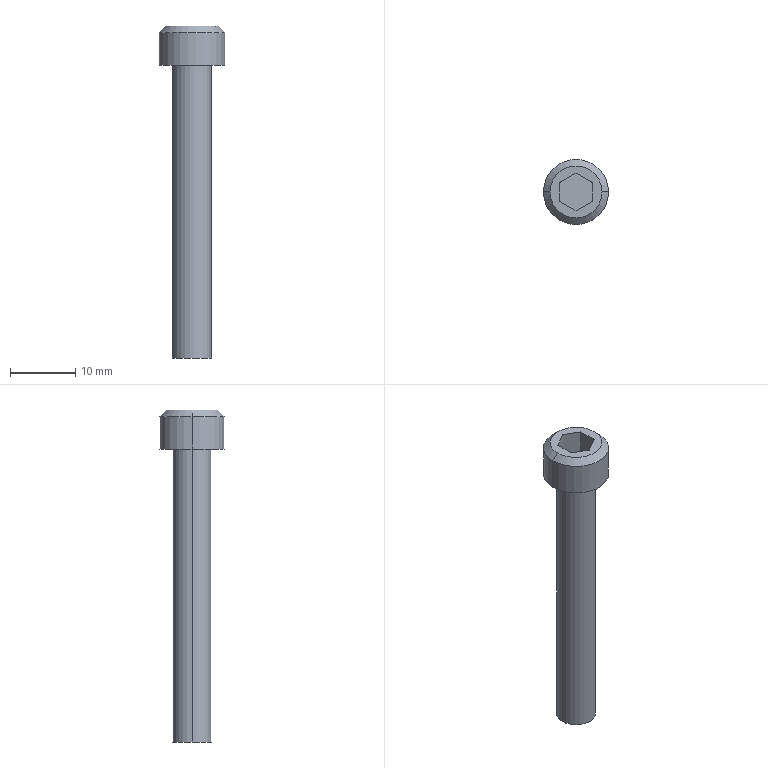Part | SolidWorks | features ICE 2, Chamfer 1, Extrusion 1 | 1 solid | 16 faces | box 10 x 10 x 51 mm | volume 1642 mm3 | plane 10 | cylinder 4 | cone 2 | commonest cylinder face diameters 6 x2 10 x2
STEP:
#1=CARTESIAN_POINT('',(-3.,0.,-45.));
#2=VERTEX_POINT('',#1);
#3=CARTESIAN_POINT('',(3.,0.,-45.));
#4=VERTEX_POINT('',#3);
#5=CARTESIAN_POINT('',(0.,0.,-45.));
#6=DIRECTION('',(0.,0.,-1.));
#7=DIRECTION('',(-1.,0.,0.));
#8=AXIS2_PLACEMENT_3D('',#5,#6,#7);
#9=CIRCLE('',#8,3.);
#10=EDGE_CURVE('',#2,#4,#9,.T.);
#11=ORIENTED_EDGE('',*,*,#10,.F.);
#12=CARTESIAN_POINT('',(-3.,0.,0.));
#13=VERTEX_POINT('',#12);
#14=CARTESIAN_POINT('',(-3.,0.,-45.));
#15=DIRECTION('',(0.,0.,1.));
#16=VECTOR('',#15,1000.);
#17=LINE('',#14,#16);
#18=EDGE_CURVE('',#2,#13,#17,.T.);
#19=ORIENTED_EDGE('',*,*,#18,.T.);
#20=CARTESIAN_POINT('',(3.,0.,0.));
#21=VERTEX_POINT('',#20);
#22=CARTESIAN_POINT('',(0.,0.,0.));
#23=DIRECTION('',(0.,0.,-1.));
#24=DIRECTION('',(1.,0.,0.));
#25=AXIS2_PLACEMENT_3D('',#22,#23,#24);
#26=CIRCLE('',#25,3.);
#27=EDGE_CURVE('',#13,#21,#26,.T.);
#28=ORIENTED_EDGE('',*,*,#27,.T.);
#29=CARTESIAN_POINT('',(3.,0.,-45.));
#30=DIRECTION('',(0.,0.,1.));
#31=VECTOR('',#30,1000.);
#32=LINE('',#29,#31);
#33=EDGE_CURVE('',#4,#21,#32,.T.);
#34=ORIENTED_EDGE('',*,*,#33,.F.);
#35=EDGE_LOOP('',(#11,#19,#28,#34));
#36=FACE_OUTER_BOUND('',#35,.T.);
#37=CARTESIAN_POINT('',(0.,0.,-45.));
#38=DIRECTION('',(0.,0.,1.));
#39=DIRECTION('',(1.,0.,0.));
#40=AXIS2_PLACEMENT_3D('',#37,#38,#39);
#41=CYLINDRICAL_SURFACE('',#40,3.);
#42=ADVANCED_FACE('',(#36),#41,.T.);
#43=CARTESIAN_POINT('',(4.,0.,6.));
#44=VERTEX_POINT('',#43);
#45=CARTESIAN_POINT('',(-4.,0.,6.));
#46=VERTEX_POINT('',#45);
#47=CARTESIAN_POINT('',(0.,0.,6.));
#48=DIRECTION('',(0.,0.,1.));
#49=DIRECTION('',(1.,0.,0.));
#50=AXIS2_PLACEMENT_3D('',#47,#48,#49);
#51=CIRCLE('',#50,4.);
#52=EDGE_CURVE('',#44,#46,#51,.T.);
#53=ORIENTED_EDGE('',*,*,#52,.F.);
#54=CARTESIAN_POINT('',(5.,0.,5.));
#55=VERTEX_POINT('',#54);
#56=CARTESIAN_POINT('',(4.,0.,6.));
#57=DIRECTION('',(0.7071,0.,-0.7071));
#58=VECTOR('',#57,1000.);
#59=LINE('',#56,#58);
#60=EDGE_CURVE('',#44,#55,#59,.T.);
#61=ORIENTED_EDGE('',*,*,#60,.T.);
#62=CARTESIAN_POINT('',(-5.,0.,5.));
#63=VERTEX_POINT('',#62);
#64=CARTESIAN_POINT('',(0.,0.,5.));
#65=DIRECTION('',(0.,0.,-1.));
#66=DIRECTION('',(1.,0.,0.));
#67=AXIS2_PLACEMENT_3D('',#64,#65,#66);
#68=CIRCLE('',#67,5.);
#69=EDGE_CURVE('',#63,#55,#68,.T.);
#70=ORIENTED_EDGE('',*,*,#69,.F.);
#71=CARTESIAN_POINT('',(-4.,0.,6.));
#72=DIRECTION('',(-0.7071,0.,-0.7071));
#73=VECTOR('',#72,1000.);
#74=LINE('',#71,#73);
#75=EDGE_CURVE('',#46,#63,#74,.T.);
#76=ORIENTED_EDGE('',*,*,#75,.F.);
#77=EDGE_LOOP('',(#53,#61,#70,#76));
#78=FACE_OUTER_BOUND('',#77,.T.);
#79=CARTESIAN_POINT('',(0.,0.,6.));
#80=DIRECTION('',(0.,0.,-1.));
#81=DIRECTION('',(-1.,0.,0.));
#82=AXIS2_PLACEMENT_3D('',#79,#80,#81);
#83=CONICAL_SURFACE('',#82,4.,0.7854);
#84=ADVANCED_FACE('',(#78),#83,.T.);
#85=ORIENTED_EDGE('',*,*,#69,.T.);
#86=CARTESIAN_POINT('',(5.,0.,0.));
#87=VERTEX_POINT('',#86);
#88=CARTESIAN_POINT('',(5.,0.,6.));
#89=DIRECTION('',(0.,0.,-1.));
#90=VECTOR('',#89,1000.);
#91=LINE('',#88,#90);
#92=EDGE_CURVE('',#55,#87,#91,.T.);
#93=ORIENTED_EDGE('',*,*,#92,.T.);
#94=CARTESIAN_POINT('',(-5.,0.,0.));
#95=VERTEX_POINT('',#94);
#96=CARTESIAN_POINT('',(0.,0.,0.));
#97=DIRECTION('',(0.,0.,1.));
#98=DIRECTION('',(1.,0.,0.));
#99=AXIS2_PLACEMENT_3D('',#96,#97,#98);
#100=CIRCLE('',#99,5.);
#101=EDGE_CURVE('',#87,#95,#100,.T.);
#102=ORIENTED_EDGE('',*,*,#101,.T.);
#103=CARTESIAN_POINT('',(-5.,0.,6.));
#104=DIRECTION('',(0.,0.,-1.));
#105=VECTOR('',#104,1000.);
#106=LINE('',#103,#105);
#107=EDGE_CURVE('',#63,#95,#106,.T.);
#108=ORIENTED_EDGE('',*,*,#107,.F.);
#109=EDGE_LOOP('',(#85,#93,#102,#108));
#110=FACE_OUTER_BOUND('',#109,.T.);
#111=CARTESIAN_POINT('',(0.,0.,6.));
#112=DIRECTION('',(0.,0.,-1.));
#113=DIRECTION('',(-1.,0.,0.));
#114=AXIS2_PLACEMENT_3D('',#111,#112,#113);
#115=CYLINDRICAL_SURFACE('',#114,5.);
#116=ADVANCED_FACE('',(#110),#115,.T.);
#117=CARTESIAN_POINT('',(0.,0.,0.));
#118=DIRECTION('',(0.,0.,1.));
#119=DIRECTION('',(1.,0.,0.));
#120=AXIS2_PLACEMENT_3D('',#117,#118,#119);
#121=CIRCLE('',#120,5.);
#122=EDGE_CURVE('',#95,#87,#121,.T.);
#123=ORIENTED_EDGE('',*,*,#122,.F.);
#124=ORIENTED_EDGE('',*,*,#101,.F.);
#125=EDGE_LOOP('',(#123,#124));
#126=FACE_OUTER_BOUND('',#125,.T.);
#127=CARTESIAN_POINT('',(0.,0.,0.));
#128=DIRECTION('',(0.,0.,-1.));
#129=DIRECTION('',(1.,0.,0.));
#130=AXIS2_PLACEMENT_3D('',#127,#128,#129);
#131=CIRCLE('',#130,3.);
#132=EDGE_CURVE('',#21,#13,#131,.T.);
#133=ORIENTED_EDGE('',*,*,#132,.F.);
#134=ORIENTED_EDGE('',*,*,#27,.F.);
#135=EDGE_LOOP('',(#133,#134));
#136=FACE_BOUND('',#135,.T.);
#137=CARTESIAN_POINT('',(0.,0.,0.));
#138=DIRECTION('',(0.,0.,1.));
#139=DIRECTION('',(1.,0.,0.));
#140=AXIS2_PLACEMENT_3D('',#137,#138,#139);
#141=PLANE('',#140);
#142=ADVANCED_FACE('',(#126,#136),#141,.F.);
#143=ORIENTED_EDGE('',*,*,#92,.F.);
#144=CARTESIAN_POINT('',(0.,0.,5.));
#145=DIRECTION('',(0.,0.,-1.));
#146=DIRECTION('',(1.,0.,0.));
#147=AXIS2_PLACEMENT_3D('',#144,#145,#146);
#148=CIRCLE('',#147,5.);
#149=EDGE_CURVE('',#55,#63,#148,.T.);
#150=ORIENTED_EDGE('',*,*,#149,.T.);
#151=ORIENTED_EDGE('',*,*,#107,.T.);
#152=ORIENTED_EDGE('',*,*,#122,.T.);
#153=EDGE_LOOP('',(#143,#150,#151,#152));
#154=FACE_OUTER_BOUND('',#153,.T.);
#155=CARTESIAN_POINT('',(0.,0.,6.));
#156=DIRECTION('',(0.,0.,-1.));
#157=DIRECTION('',(-1.,0.,0.));
#158=AXIS2_PLACEMENT_3D('',#155,#156,#157);
#159=CYLINDRICAL_SURFACE('',#158,5.);
#160=ADVANCED_FACE('',(#154),#159,.T.);
#161=CARTESIAN_POINT('',(0.,0.,6.));
#162=DIRECTION('',(0.,0.,1.));
#163=DIRECTION('',(1.,0.,0.));
#164=AXIS2_PLACEMENT_3D('',#161,#162,#163);
#165=CIRCLE('',#164,4.);
#166=EDGE_CURVE('',#46,#44,#165,.T.);
#167=ORIENTED_EDGE('',*,*,#166,.T.);
#168=ORIENTED_EDGE('',*,*,#52,.T.);
#169=EDGE_LOOP('',(#167,#168));
#170=FACE_OUTER_BOUND('',#169,.T.);
#171=CARTESIAN_POINT('',(2.5,1.443,6.));
#172=VERTEX_POINT('',#171);
#173=CARTESIAN_POINT('',(0.,2.887,6.));
#174=VERTEX_POINT('',#173);
#175=CARTESIAN_POINT('',(2.5,1.443,6.));
#176=DIRECTION('',(-0.866,0.5,0.));
#177=VECTOR('',#176,1000.);
#178=LINE('',#175,#177);
#179=EDGE_CURVE('',#172,#174,#178,.T.);
#180=ORIENTED_EDGE('',*,*,#179,.F.);
#181=CARTESIAN_POINT('',(2.5,-1.443,6.));
#182=VERTEX_POINT('',#181);
#183=CARTESIAN_POINT('',(2.5,-1.443,6.));
#184=DIRECTION('',(0.,1.,0.));
#185=VECTOR('',#184,1000.);
#186=LINE('',#183,#185);
#187=EDGE_CURVE('',#182,#172,#186,.T.);
#188=ORIENTED_EDGE('',*,*,#187,.F.);
#189=CARTESIAN_POINT('',(0.,-2.887,6.));
#190=VERTEX_POINT('',#189);
#191=CARTESIAN_POINT('',(0.,-2.887,6.));
#192=DIRECTION('',(0.866,0.5,0.));
#193=VECTOR('',#192,1000.);
#194=LINE('',#191,#193);
#195=EDGE_CURVE('',#190,#182,#194,.T.);
#196=ORIENTED_EDGE('',*,*,#195,.F.);
#197=CARTESIAN_POINT('',(-2.5,-1.443,6.));
#198=VERTEX_POINT('',#197);
#199=CARTESIAN_POINT('',(-2.5,-1.443,6.));
#200=DIRECTION('',(0.866,-0.5,0.));
#201=VECTOR('',#200,1000.);
#202=LINE('',#199,#201);
#203=EDGE_CURVE('',#198,#190,#202,.T.);
#204=ORIENTED_EDGE('',*,*,#203,.F.);
#205=CARTESIAN_POINT('',(-2.5,1.443,6.));
#206=VERTEX_POINT('',#205);
#207=CARTESIAN_POINT('',(-2.5,1.443,6.));
#208=DIRECTION('',(0.,-1.,0.));
#209=VECTOR('',#208,1000.);
#210=LINE('',#207,#209);
#211=EDGE_CURVE('',#206,#198,#210,.T.);
#212=ORIENTED_EDGE('',*,*,#211,.F.);
#213=CARTESIAN_POINT('',(0.,2.887,6.));
#214=DIRECTION('',(-0.866,-0.5,0.));
#215=VECTOR('',#214,1000.);
#216=LINE('',#213,#215);
#217=EDGE_CURVE('',#174,#206,#216,.T.);
#218=ORIENTED_EDGE('',*,*,#217,.F.);
#219=EDGE_LOOP('',(#180,#188,#196,#204,#212,#218));
#220=FACE_BOUND('',#219,.T.);
#221=CARTESIAN_POINT('',(0.,0.,6.));
#222=DIRECTION('',(0.,0.,1.));
#223=DIRECTION('',(1.,0.,0.));
#224=AXIS2_PLACEMENT_3D('',#221,#222,#223);
#225=PLANE('',#224);
#226=ADVANCED_FACE('',(#170,#220),#225,.T.);
#227=ORIENTED_EDGE('',*,*,#179,.T.);
#228=CARTESIAN_POINT('',(0.,2.887,2.));
#229=VERTEX_POINT('',#228);
#230=CARTESIAN_POINT('',(0.,2.887,2.));
#231=DIRECTION('',(0.,0.,1.));
#232=VECTOR('',#231,1000.);
#233=LINE('',#230,#232);
#234=EDGE_CURVE('',#229,#174,#233,.T.);
#235=ORIENTED_EDGE('',*,*,#234,.F.);
#236=CARTESIAN_POINT('',(2.5,1.443,2.));
#237=VERTEX_POINT('',#236);
#238=CARTESIAN_POINT('',(2.5,1.443,2.));
#239=DIRECTION('',(-0.866,0.5,0.));
#240=VECTOR('',#239,1000.);
#241=LINE('',#238,#240);
#242=EDGE_CURVE('',#237,#229,#241,.T.);
#243=ORIENTED_EDGE('',*,*,#242,.F.);
#244=CARTESIAN_POINT('',(2.5,1.443,2.));
#245=DIRECTION('',(0.,0.,1.));
#246=VECTOR('',#245,1000.);
#247=LINE('',#244,#246);
#248=EDGE_CURVE('',#237,#172,#247,.T.);
#249=ORIENTED_EDGE('',*,*,#248,.T.);
#250=EDGE_LOOP('',(#227,#235,#243,#249));
#251=FACE_OUTER_BOUND('',#250,.T.);
#252=CARTESIAN_POINT('',(2.5,1.443,2.));
#253=DIRECTION('',(0.5,0.866,0.));
#254=DIRECTION('',(-0.866,0.5,0.));
#255=AXIS2_PLACEMENT_3D('',#252,#253,#254);
#256=PLANE('',#255);
#257=ADVANCED_FACE('',(#251),#256,.F.);
#258=ORIENTED_EDGE('',*,*,#187,.T.);
#259=ORIENTED_EDGE('',*,*,#248,.F.);
#260=CARTESIAN_POINT('',(2.5,-1.443,2.));
#261=VERTEX_POINT('',#260);
#262=CARTESIAN_POINT('',(2.5,-1.443,2.));
#263=DIRECTION('',(0.,1.,0.));
#264=VECTOR('',#263,1000.);
#265=LINE('',#262,#264);
#266=EDGE_CURVE('',#261,#237,#265,.T.);
#267=ORIENTED_EDGE('',*,*,#266,.F.);
#268=CARTESIAN_POINT('',(2.5,-1.443,2.));
#269=DIRECTION('',(0.,0.,1.));
#270=VECTOR('',#269,1000.);
#271=LINE('',#268,#270);
#272=EDGE_CURVE('',#261,#182,#271,.T.);
#273=ORIENTED_EDGE('',*,*,#272,.T.);
#274=EDGE_LOOP('',(#258,#259,#267,#273));
#275=FACE_OUTER_BOUND('',#274,.T.);
#276=CARTESIAN_POINT('',(2.5,-1.443,2.));
#277=DIRECTION('',(1.,0.,0.));
#278=DIRECTION('',(0.,1.,0.));
#279=AXIS2_PLACEMENT_3D('',#276,#277,#278);
#280=PLANE('',#279);
#281=ADVANCED_FACE('',(#275),#280,.F.);
#282=ORIENTED_EDGE('',*,*,#195,.T.);
#283=ORIENTED_EDGE('',*,*,#272,.F.);
#284=CARTESIAN_POINT('',(0.,-2.887,2.));
#285=VERTEX_POINT('',#284);
#286=CARTESIAN_POINT('',(0.,-2.887,2.));
#287=DIRECTION('',(0.866,0.5,0.));
#288=VECTOR('',#287,1000.);
#289=LINE('',#286,#288);
#290=EDGE_CURVE('',#285,#261,#289,.T.);
#291=ORIENTED_EDGE('',*,*,#290,.F.);
#292=CARTESIAN_POINT('',(0.,-2.887,2.));
#293=DIRECTION('',(0.,0.,1.));
#294=VECTOR('',#293,1000.);
#295=LINE('',#292,#294);
#296=EDGE_CURVE('',#285,#190,#295,.T.);
#297=ORIENTED_EDGE('',*,*,#296,.T.);
#298=EDGE_LOOP('',(#282,#283,#291,#297));
#299=FACE_OUTER_BOUND('',#298,.T.);
#300=CARTESIAN_POINT('',(0.,-2.887,2.));
#301=DIRECTION('',(0.5,-0.866,0.));
#302=DIRECTION('',(0.866,0.5,0.));
#303=AXIS2_PLACEMENT_3D('',#300,#301,#302);
#304=PLANE('',#303);
#305=ADVANCED_FACE('',(#299),#304,.F.);
#306=ORIENTED_EDGE('',*,*,#203,.T.);
#307=ORIENTED_EDGE('',*,*,#296,.F.);
#308=CARTESIAN_POINT('',(-2.5,-1.443,2.));
#309=VERTEX_POINT('',#308);
#310=CARTESIAN_POINT('',(-2.5,-1.443,2.));
#311=DIRECTION('',(0.866,-0.5,0.));
#312=VECTOR('',#311,1000.);
#313=LINE('',#310,#312);
#314=EDGE_CURVE('',#309,#285,#313,.T.);
#315=ORIENTED_EDGE('',*,*,#314,.F.);
#316=CARTESIAN_POINT('',(-2.5,-1.443,2.));
#317=DIRECTION('',(0.,0.,1.));
#318=VECTOR('',#317,1000.);
#319=LINE('',#316,#318);
#320=EDGE_CURVE('',#309,#198,#319,.T.);
#321=ORIENTED_EDGE('',*,*,#320,.T.);
#322=EDGE_LOOP('',(#306,#307,#315,#321));
#323=FACE_OUTER_BOUND('',#322,.T.);
#324=CARTESIAN_POINT('',(-2.5,-1.443,2.));
#325=DIRECTION('',(-0.5,-0.866,0.));
#326=DIRECTION('',(0.866,-0.5,0.));
#327=AXIS2_PLACEMENT_3D('',#324,#325,#326);
#328=PLANE('',#327);
#329=ADVANCED_FACE('',(#323),#328,.F.);
#330=ORIENTED_EDGE('',*,*,#211,.T.);
#331=ORIENTED_EDGE('',*,*,#320,.F.);
#332=CARTESIAN_POINT('',(-2.5,1.443,2.));
#333=VERTEX_POINT('',#332);
#334=CARTESIAN_POINT('',(-2.5,1.443,2.));
#335=DIRECTION('',(0.,-1.,0.));
#336=VECTOR('',#335,1000.);
#337=LINE('',#334,#336);
#338=EDGE_CURVE('',#333,#309,#337,.T.);
#339=ORIENTED_EDGE('',*,*,#338,.F.);
#340=CARTESIAN_POINT('',(-2.5,1.443,2.));
#341=DIRECTION('',(0.,0.,1.));
#342=VECTOR('',#341,1000.);
#343=LINE('',#340,#342);
#344=EDGE_CURVE('',#333,#206,#343,.T.);
#345=ORIENTED_EDGE('',*,*,#344,.T.);
#346=EDGE_LOOP('',(#330,#331,#339,#345));
#347=FACE_OUTER_BOUND('',#346,.T.);
#348=CARTESIAN_POINT('',(-2.5,1.443,2.));
#349=DIRECTION('',(-1.,0.,0.));
#350=DIRECTION('',(0.,0.,1.));
#351=AXIS2_PLACEMENT_3D('',#348,#349,#350);
#352=PLANE('',#351);
#353=ADVANCED_FACE('',(#347),#352,.F.);
#354=ORIENTED_EDGE('',*,*,#217,.T.);
#355=ORIENTED_EDGE('',*,*,#344,.F.);
#356=CARTESIAN_POINT('',(0.,2.887,2.));
#357=DIRECTION('',(-0.866,-0.5,0.));
#358=VECTOR('',#357,1000.);
#359=LINE('',#356,#358);
#360=EDGE_CURVE('',#229,#333,#359,.T.);
#361=ORIENTED_EDGE('',*,*,#360,.F.);
#362=ORIENTED_EDGE('',*,*,#234,.T.);
#363=EDGE_LOOP('',(#354,#355,#361,#362));
#364=FACE_OUTER_BOUND('',#363,.T.);
#365=CARTESIAN_POINT('',(0.,2.887,2.));
#366=DIRECTION('',(-0.5,0.866,0.));
#367=DIRECTION('',(-0.866,-0.5,0.));
#368=AXIS2_PLACEMENT_3D('',#365,#366,#367);
#369=PLANE('',#368);
#370=ADVANCED_FACE('',(#364),#369,.F.);
#371=ORIENTED_EDGE('',*,*,#242,.T.);
#372=ORIENTED_EDGE('',*,*,#360,.T.);
#373=ORIENTED_EDGE('',*,*,#338,.T.);
#374=ORIENTED_EDGE('',*,*,#314,.T.);
#375=ORIENTED_EDGE('',*,*,#290,.T.);
#376=ORIENTED_EDGE('',*,*,#266,.T.);
#377=EDGE_LOOP('',(#371,#372,#373,#374,#375,#376));
#378=FACE_OUTER_BOUND('',#377,.T.);
#379=CARTESIAN_POINT('',(0.,0.,2.));
#380=DIRECTION('',(0.,0.,1.));
#381=DIRECTION('',(1.,0.,0.));
#382=AXIS2_PLACEMENT_3D('',#379,#380,#381);
#383=PLANE('',#382);
#384=ADVANCED_FACE('',(#378),#383,.T.);
#385=ORIENTED_EDGE('',*,*,#60,.F.);
#386=ORIENTED_EDGE('',*,*,#166,.F.);
#387=ORIENTED_EDGE('',*,*,#75,.T.);
#388=ORIENTED_EDGE('',*,*,#149,.F.);
#389=EDGE_LOOP('',(#385,#386,#387,#388));
#390=FACE_OUTER_BOUND('',#389,.T.);
#391=CARTESIAN_POINT('',(0.,0.,6.));
#392=DIRECTION('',(0.,0.,-1.));
#393=DIRECTION('',(-1.,0.,0.));
#394=AXIS2_PLACEMENT_3D('',#391,#392,#393);
#395=CONICAL_SURFACE('',#394,4.,0.7854);
#396=ADVANCED_FACE('',(#390),#395,.T.);
#397=ORIENTED_EDGE('',*,*,#18,.F.);
#398=CARTESIAN_POINT('',(0.,0.,-45.));
#399=DIRECTION('',(0.,0.,-1.));
#400=DIRECTION('',(-1.,0.,0.));
#401=AXIS2_PLACEMENT_3D('',#398,#399,#400);
#402=CIRCLE('',#401,3.);
#403=EDGE_CURVE('',#4,#2,#402,.T.);
#404=ORIENTED_EDGE('',*,*,#403,.F.);
#405=ORIENTED_EDGE('',*,*,#33,.T.);
#406=ORIENTED_EDGE('',*,*,#132,.T.);
#407=EDGE_LOOP('',(#397,#404,#405,#406));
#408=FACE_OUTER_BOUND('',#407,.T.);
#409=CARTESIAN_POINT('',(0.,0.,-45.));
#410=DIRECTION('',(0.,0.,1.));
#411=DIRECTION('',(1.,0.,0.));
#412=AXIS2_PLACEMENT_3D('',#409,#410,#411);
#413=CYLINDRICAL_SURFACE('',#412,3.);
#414=ADVANCED_FACE('',(#408),#413,.T.);
#415=ORIENTED_EDGE('',*,*,#403,.T.);
#416=ORIENTED_EDGE('',*,*,#10,.T.);
#417=EDGE_LOOP('',(#415,#416));
#418=FACE_OUTER_BOUND('',#417,.T.);
#419=CARTESIAN_POINT('',(0.,0.,-45.));
#420=DIRECTION('',(0.,0.,-1.));
#421=DIRECTION('',(-1.,0.,0.));
#422=AXIS2_PLACEMENT_3D('',#419,#420,#421);
#423=PLANE('',#422);
#424=ADVANCED_FACE('',(#418),#423,.T.);
#425=CLOSED_SHELL('',(#42,#84,#116,#142,#160,#226,#257,#281,#305,#329,#353,#370,#384,#396,#414,#424));
#426=MANIFOLD_SOLID_BREP('',#425);
#427=CARTESIAN_POINT('',(0.,0.,0.));
#428=DIRECTION('',(0.,0.,1.));
#429=DIRECTION('',(1.,0.,0.));
#430=AXIS2_PLACEMENT_3D('',#427,#428,#429);
#431=(LENGTH_UNIT()NAMED_UNIT(*)SI_UNIT(.MILLI.,.METRE.));
#432=UNCERTAINTY_MEASURE_WITH_UNIT(LENGTH_MEASURE(0.00001),#431,'','');
#433=(NAMED_UNIT(*)PLANE_ANGLE_UNIT()SI_UNIT($,.RADIAN.));
#434=(NAMED_UNIT(*)SI_UNIT($,.STERADIAN.)SOLID_ANGLE_UNIT());
#435=(GEOMETRIC_REPRESENTATION_CONTEXT(3)GLOBAL_UNCERTAINTY_ASSIGNED_CONTEXT((#432))GLOBAL_UNIT_ASSIGNED_CONTEXT((#431,#433,#434))REPRESENTATION_CONTEXT('',''));
#436=ADVANCED_BREP_SHAPE_REPRESENTATION('',(#426,#430),#435);